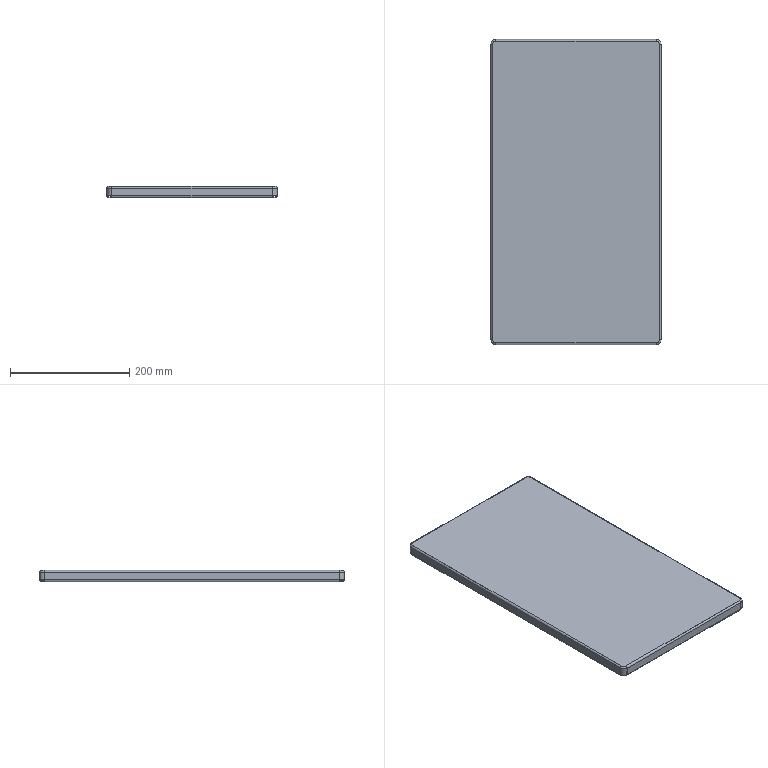Part | STEP file | Front small door panel V1.201001 | 1 solid | 114 faces | box 285 x 511 x 19 mm | volume 277788 mm3 | plane 82 | cylinder 24 | torus 8 | commonest cylinder face diameters 3 x8 6 x8 13 x4 16 x4